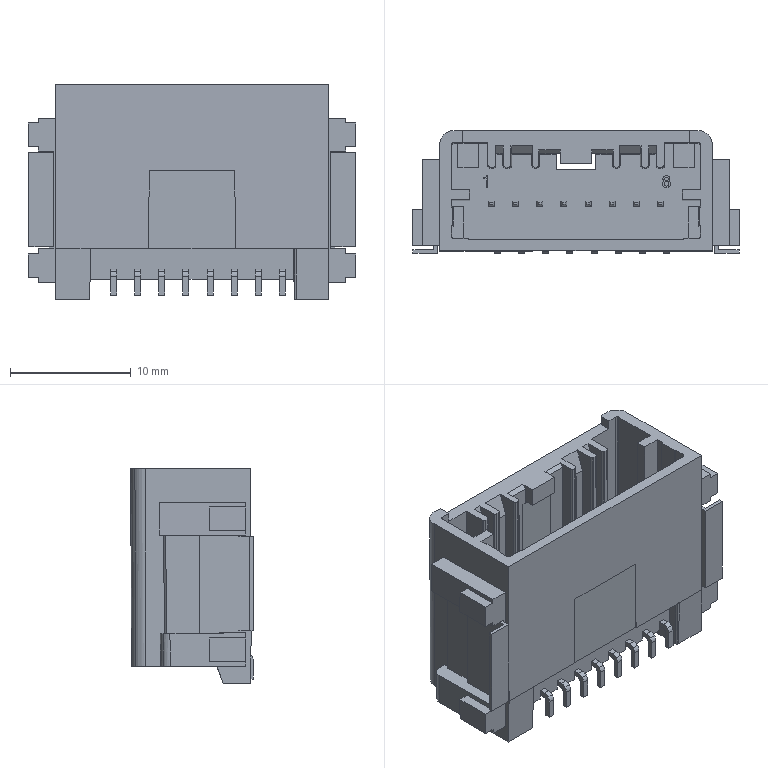Part | NX | features BREP 1 | 1 solid | 647 faces | box 27.19 x 10.174 x 17.8 mm | volume 1535 mm3 | plane 511 | cylinder 134 | spline 2 | commonest cylinder face diameters 0.4 x58 1.6 x20 0.6 x16 0.8 x16 1.2 x16 2.4 x4